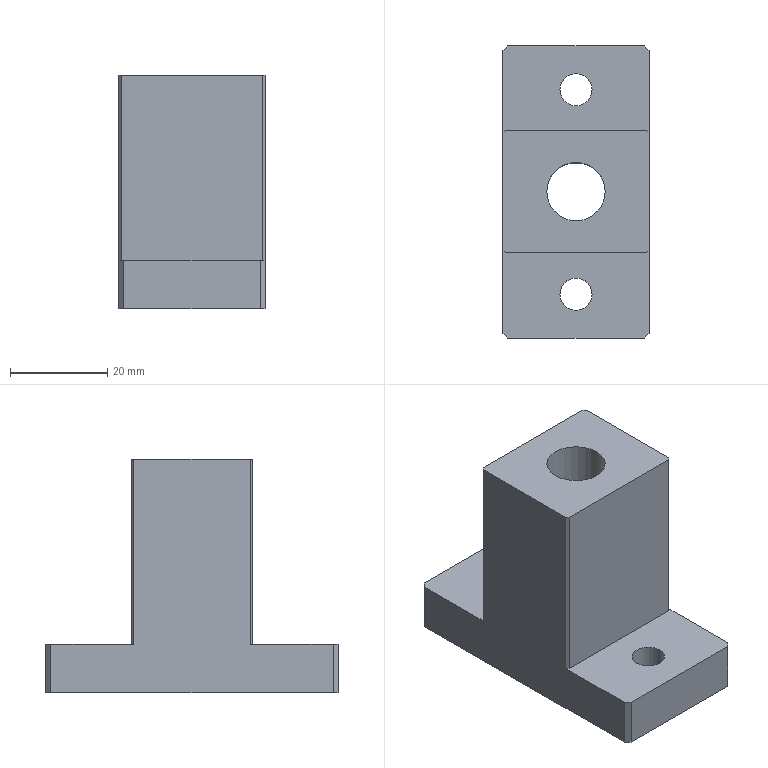NC program | NX | posted with a generic post | part box 30 x 60 x 48 mm
Lines 1 to 18 of 6343:
N10 G17 G21 G94 G90
(PLANAR_MILL , TOOL : D50面刀)
N12 T01 M6
N14 G53
N16 G17 G0 G90 X59. Y0. S1600 M3
N18 G43 Z20. H1
N20 Z3.
N22 G94 G1 Z0. F800.
N24 X29.
N26 X-29.
N28 X-59.
N30 Z3.
N32 G0 Z20.
N34 M5